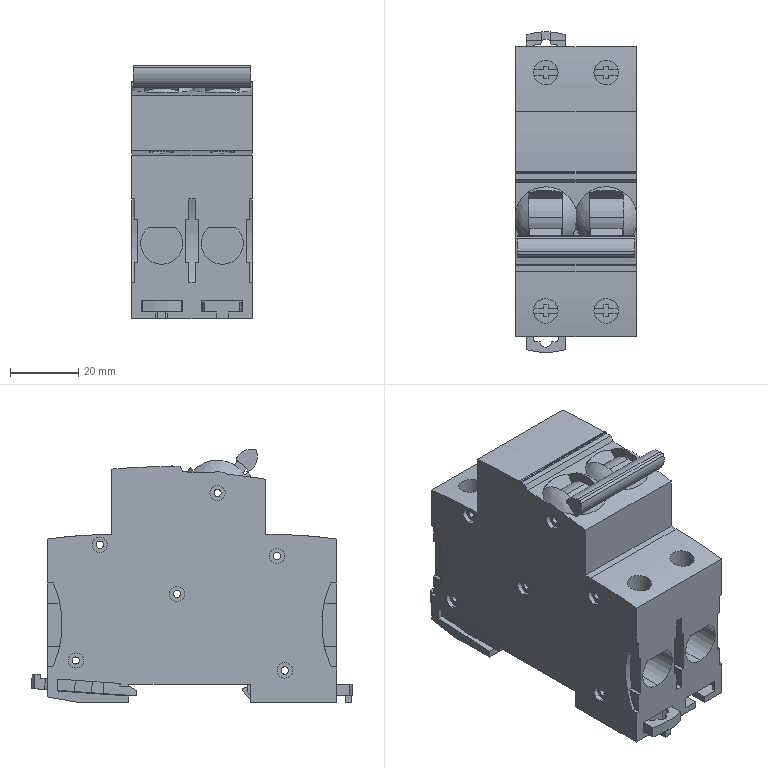Part | STEP file | Miniature circuit breaker IC65N-2P-C16A | 8 solids | 502 faces | box 35.4 x 93.9 x 74.3 mm | volume 159125 mm3 | plane 381 | cylinder 119 | spline 2 | commonest cylinder face diameters 4.5 x24 2.1 x16 7.2 x16 12.299 x8 2 x7 60 x6